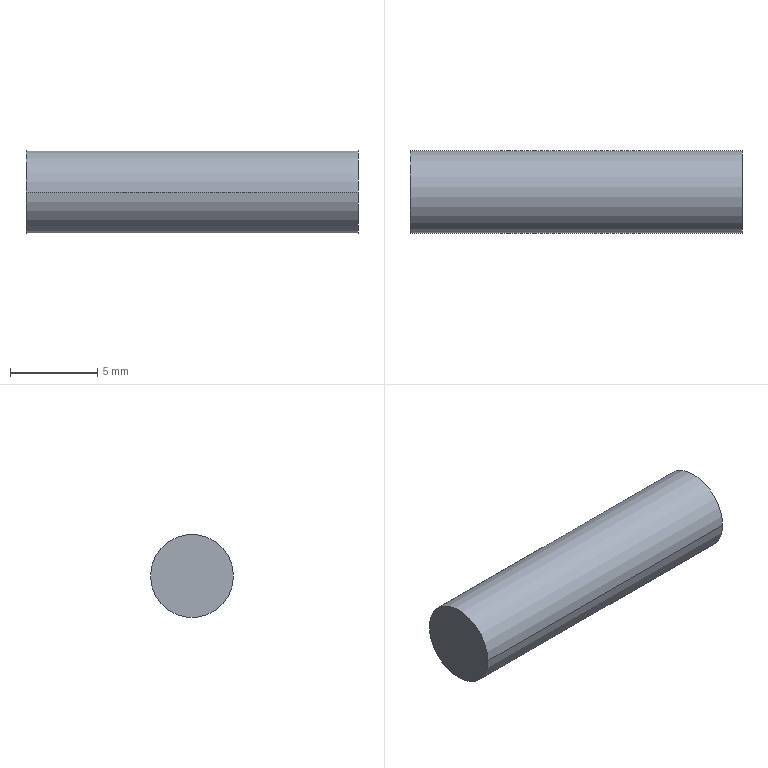Part | NX | features BREP 1 | 1 solid | 4 faces | box 19.05 x 4.763 x 4.763 mm | volume 339.355 mm3 | plane 2 | cylinder 2 | commonest cylinder face diameters 4.763 x2
STEP:
#1=CARTESIAN_POINT('',(0.,2.381,0.));
#2=VERTEX_POINT('',#1);
#3=CARTESIAN_POINT('',(0.,-2.381,0.));
#4=VERTEX_POINT('',#3);
#5=CARTESIAN_POINT('',(0.,0.,0.));
#6=DIRECTION('',(1.,0.,0.));
#7=DIRECTION('',(0.,1.,0.));
#8=AXIS2_PLACEMENT_3D('',#5,#6,#7);
#9=CIRCLE('',#8,2.381);
#10=EDGE_CURVE('',#2,#4,#9,.T.);
#11=ORIENTED_EDGE('',*,*,#10,.F.);
#12=CARTESIAN_POINT('',(0.,0.,0.));
#13=DIRECTION('',(1.,0.,0.));
#14=DIRECTION('',(0.,-1.,0.));
#15=AXIS2_PLACEMENT_3D('',#12,#13,#14);
#16=CIRCLE('',#15,2.381);
#17=EDGE_CURVE('',#4,#2,#16,.T.);
#18=ORIENTED_EDGE('',*,*,#17,.F.);
#19=EDGE_LOOP('',(#11,#18));
#20=FACE_BOUND('',#19,.T.);
#21=CARTESIAN_POINT('',(0.,0.,0.));
#22=DIRECTION('',(1.,0.,0.));
#23=DIRECTION('',(0.,1.,0.));
#24=AXIS2_PLACEMENT_3D('',#21,#22,#23);
#25=PLANE('',#24);
#26=ADVANCED_FACE('',(#20),#25,.F.);
#27=CARTESIAN_POINT('',(19.05,2.381,0.));
#28=VERTEX_POINT('',#27);
#29=CARTESIAN_POINT('',(0.,2.381,0.));
#30=DIRECTION('',(1.,0.,0.));
#31=VECTOR('',#30,1000.);
#32=LINE('',#29,#31);
#33=EDGE_CURVE('',#28,#2,#32,.F.);
#34=ORIENTED_EDGE('',*,*,#33,.F.);
#35=CARTESIAN_POINT('',(19.05,-2.381,0.));
#36=VERTEX_POINT('',#35);
#37=CARTESIAN_POINT('',(19.05,0.,0.));
#38=DIRECTION('',(1.,0.,0.));
#39=DIRECTION('',(0.,-1.,0.));
#40=AXIS2_PLACEMENT_3D('',#37,#38,#39);
#41=CIRCLE('',#40,2.381);
#42=EDGE_CURVE('',#36,#28,#41,.T.);
#43=ORIENTED_EDGE('',*,*,#42,.F.);
#44=CARTESIAN_POINT('',(0.,-2.381,0.));
#45=DIRECTION('',(1.,0.,0.));
#46=VECTOR('',#45,1000.);
#47=LINE('',#44,#46);
#48=EDGE_CURVE('',#36,#4,#47,.F.);
#49=ORIENTED_EDGE('',*,*,#48,.T.);
#50=ORIENTED_EDGE('',*,*,#17,.T.);
#51=EDGE_LOOP('',(#34,#43,#49,#50));
#52=FACE_BOUND('',#51,.T.);
#53=CARTESIAN_POINT('',(0.,0.,0.));
#54=DIRECTION('',(1.,0.,0.));
#55=DIRECTION('',(0.,-1.,0.));
#56=AXIS2_PLACEMENT_3D('',#53,#54,#55);
#57=CYLINDRICAL_SURFACE('',#56,2.381);
#58=ADVANCED_FACE('',(#52),#57,.T.);
#59=ORIENTED_EDGE('',*,*,#48,.F.);
#60=CARTESIAN_POINT('',(19.05,0.,0.));
#61=DIRECTION('',(1.,0.,0.));
#62=DIRECTION('',(0.,1.,0.));
#63=AXIS2_PLACEMENT_3D('',#60,#61,#62);
#64=CIRCLE('',#63,2.381);
#65=EDGE_CURVE('',#28,#36,#64,.T.);
#66=ORIENTED_EDGE('',*,*,#65,.F.);
#67=ORIENTED_EDGE('',*,*,#33,.T.);
#68=ORIENTED_EDGE('',*,*,#10,.T.);
#69=EDGE_LOOP('',(#59,#66,#67,#68));
#70=FACE_BOUND('',#69,.T.);
#71=CARTESIAN_POINT('',(0.,0.,0.));
#72=DIRECTION('',(1.,0.,0.));
#73=DIRECTION('',(0.,-1.,0.));
#74=AXIS2_PLACEMENT_3D('',#71,#72,#73);
#75=CYLINDRICAL_SURFACE('',#74,2.381);
#76=ADVANCED_FACE('',(#70),#75,.T.);
#77=ORIENTED_EDGE('',*,*,#65,.T.);
#78=ORIENTED_EDGE('',*,*,#42,.T.);
#79=EDGE_LOOP('',(#77,#78));
#80=FACE_BOUND('',#79,.T.);
#81=CARTESIAN_POINT('',(19.05,0.,0.));
#82=DIRECTION('',(1.,0.,0.));
#83=DIRECTION('',(0.,1.,0.));
#84=AXIS2_PLACEMENT_3D('',#81,#82,#83);
#85=PLANE('',#84);
#86=ADVANCED_FACE('',(#80),#85,.T.);
#87=CLOSED_SHELL('',(#26,#58,#76,#86));
#88=MANIFOLD_SOLID_BREP('',#87);
#89=(LENGTH_UNIT()NAMED_UNIT(*)SI_UNIT(.MILLI.,.METRE.));
#90=UNCERTAINTY_MEASURE_WITH_UNIT(LENGTH_MEASURE(0.00001),#89,'','');
#91=(NAMED_UNIT(*)PLANE_ANGLE_UNIT()SI_UNIT($,.RADIAN.));
#92=(NAMED_UNIT(*)SI_UNIT($,.STERADIAN.)SOLID_ANGLE_UNIT());
#93=(GEOMETRIC_REPRESENTATION_CONTEXT(3)GLOBAL_UNCERTAINTY_ASSIGNED_CONTEXT((#90))GLOBAL_UNIT_ASSIGNED_CONTEXT((#89,#91,#92))REPRESENTATION_CONTEXT('',''));
#94=ADVANCED_BREP_SHAPE_REPRESENTATION('',(#88),#93);